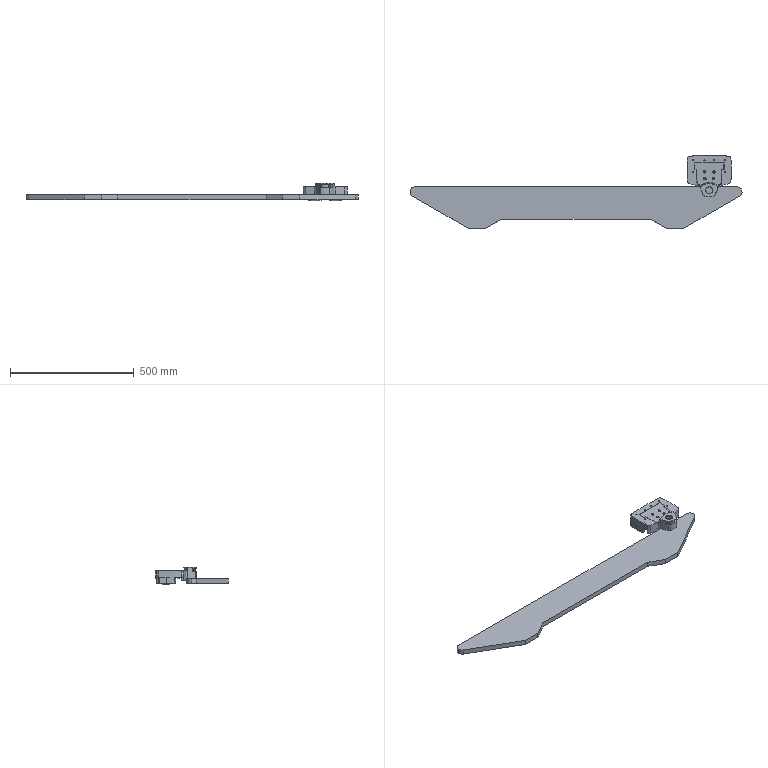Part | SolidWorks | features BaseBody 1, Fillet 1, ICE 1, Scale 1 | 1 solid | 359 faces | box 1341 x 293.909 x 70 mm | volume 4218452 mm3 | plane 176 | cylinder 138 | torus 28 | cone 17 | commonest cylinder face diameters 4.55 x16 7 x16 11.2 x10 2.8 x8 9.8 x8 28 x8